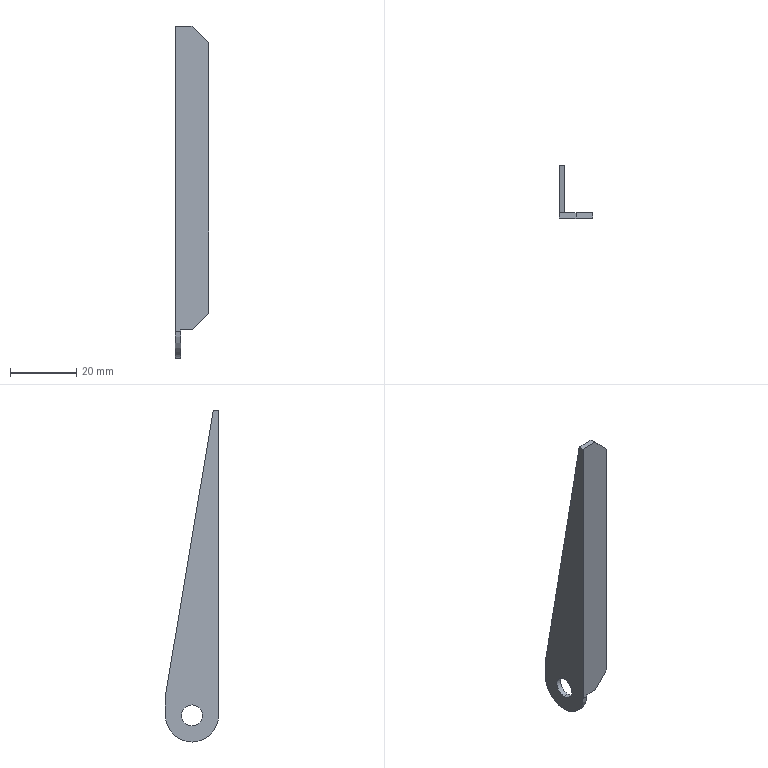Part | SolidWorks | features BaseBody 1 | 1 solid | 15 faces | box 10 x 16 x 100 mm | volume 2664 mm3 | plane 11 | cylinder 4 | commonest cylinder face diameters 6.35 x2 16 x2
STEP:
#1=CARTESIAN_POINT('',(0.,8.,4.825));
#2=VERTEX_POINT('',#1);
#3=CARTESIAN_POINT('',(0.,8.,11.175));
#4=VERTEX_POINT('',#3);
#5=CARTESIAN_POINT('',(0.,8.,8.));
#6=DIRECTION('',(-1.,0.,0.));
#7=DIRECTION('',(0.,0.,-1.));
#8=AXIS2_PLACEMENT_3D('',#5,#6,#7);
#9=CIRCLE('',#8,3.175);
#10=EDGE_CURVE('',#2,#4,#9,.T.);
#11=ORIENTED_EDGE('',*,*,#10,.T.);
#12=CARTESIAN_POINT('',(1.6,8.,11.175));
#13=VERTEX_POINT('',#12);
#14=CARTESIAN_POINT('',(0.,8.,11.175));
#15=DIRECTION('',(1.,0.,0.));
#16=VECTOR('',#15,1000.);
#17=LINE('',#14,#16);
#18=EDGE_CURVE('',#4,#13,#17,.T.);
#19=ORIENTED_EDGE('',*,*,#18,.T.);
#20=CARTESIAN_POINT('',(1.6,8.,4.825));
#21=VERTEX_POINT('',#20);
#22=CARTESIAN_POINT('',(1.6,8.,8.));
#23=DIRECTION('',(1.,0.,0.));
#24=DIRECTION('',(0.,0.,-1.));
#25=AXIS2_PLACEMENT_3D('',#22,#23,#24);
#26=CIRCLE('',#25,3.175);
#27=EDGE_CURVE('',#13,#21,#26,.T.);
#28=ORIENTED_EDGE('',*,*,#27,.T.);
#29=CARTESIAN_POINT('',(0.,8.,4.825));
#30=DIRECTION('',(1.,0.,0.));
#31=VECTOR('',#30,1000.);
#32=LINE('',#29,#31);
#33=EDGE_CURVE('',#2,#21,#32,.T.);
#34=ORIENTED_EDGE('',*,*,#33,.F.);
#35=EDGE_LOOP('',(#11,#19,#28,#34));
#36=FACE_OUTER_BOUND('',#35,.T.);
#37=CARTESIAN_POINT('',(0.,8.,8.));
#38=DIRECTION('',(1.,0.,0.));
#39=DIRECTION('',(0.,0.,-1.));
#40=AXIS2_PLACEMENT_3D('',#37,#38,#39);
#41=CYLINDRICAL_SURFACE('',#40,3.175);
#42=ADVANCED_FACE('',(#36),#41,.F.);
#43=CARTESIAN_POINT('',(0.,0.,8.));
#44=VERTEX_POINT('',#43);
#45=CARTESIAN_POINT('',(0.,8.,0.));
#46=VERTEX_POINT('',#45);
#47=CARTESIAN_POINT('',(0.,8.,8.));
#48=DIRECTION('',(1.,0.,0.));
#49=DIRECTION('',(0.,0.,-1.));
#50=AXIS2_PLACEMENT_3D('',#47,#48,#49);
#51=CIRCLE('',#50,8.);
#52=EDGE_CURVE('',#44,#46,#51,.T.);
#53=ORIENTED_EDGE('',*,*,#52,.T.);
#54=CARTESIAN_POINT('',(1.6,8.,0.));
#55=VERTEX_POINT('',#54);
#56=CARTESIAN_POINT('',(0.,8.,0.));
#57=DIRECTION('',(1.,0.,0.));
#58=VECTOR('',#57,1000.);
#59=LINE('',#56,#58);
#60=EDGE_CURVE('',#46,#55,#59,.T.);
#61=ORIENTED_EDGE('',*,*,#60,.T.);
#62=CARTESIAN_POINT('',(1.6,0.,8.));
#63=VERTEX_POINT('',#62);
#64=CARTESIAN_POINT('',(1.6,8.,8.));
#65=DIRECTION('',(-1.,0.,0.));
#66=DIRECTION('',(0.,0.,-1.));
#67=AXIS2_PLACEMENT_3D('',#64,#65,#66);
#68=CIRCLE('',#67,8.);
#69=EDGE_CURVE('',#55,#63,#68,.T.);
#70=ORIENTED_EDGE('',*,*,#69,.T.);
#71=CARTESIAN_POINT('',(0.8,0.,8.));
#72=DIRECTION('',(1.,0.,0.));
#73=VECTOR('',#72,1000.);
#74=LINE('',#71,#73);
#75=EDGE_CURVE('',#44,#63,#74,.T.);
#76=ORIENTED_EDGE('',*,*,#75,.F.);
#77=EDGE_LOOP('',(#53,#61,#70,#76));
#78=FACE_OUTER_BOUND('',#77,.T.);
#79=CARTESIAN_POINT('',(0.,8.,8.));
#80=DIRECTION('',(1.,0.,0.));
#81=DIRECTION('',(0.,0.,-1.));
#82=AXIS2_PLACEMENT_3D('',#79,#80,#81);
#83=CYLINDRICAL_SURFACE('',#82,8.);
#84=ADVANCED_FACE('',(#78),#83,.T.);
#85=ORIENTED_EDGE('',*,*,#18,.F.);
#86=CARTESIAN_POINT('',(0.,8.,8.));
#87=DIRECTION('',(-1.,0.,0.));
#88=DIRECTION('',(0.,0.,-1.));
#89=AXIS2_PLACEMENT_3D('',#86,#87,#88);
#90=CIRCLE('',#89,3.175);
#91=EDGE_CURVE('',#4,#2,#90,.T.);
#92=ORIENTED_EDGE('',*,*,#91,.T.);
#93=ORIENTED_EDGE('',*,*,#33,.T.);
#94=CARTESIAN_POINT('',(1.6,8.,8.));
#95=DIRECTION('',(1.,0.,0.));
#96=DIRECTION('',(0.,0.,-1.));
#97=AXIS2_PLACEMENT_3D('',#94,#95,#96);
#98=CIRCLE('',#97,3.175);
#99=EDGE_CURVE('',#21,#13,#98,.T.);
#100=ORIENTED_EDGE('',*,*,#99,.T.);
#101=EDGE_LOOP('',(#85,#92,#93,#100));
#102=FACE_OUTER_BOUND('',#101,.T.);
#103=CARTESIAN_POINT('',(0.,8.,8.));
#104=DIRECTION('',(1.,0.,0.));
#105=DIRECTION('',(0.,0.,-1.));
#106=AXIS2_PLACEMENT_3D('',#103,#104,#105);
#107=CYLINDRICAL_SURFACE('',#106,3.175);
#108=ADVANCED_FACE('',(#102),#107,.F.);
#109=ORIENTED_EDGE('',*,*,#99,.F.);
#110=ORIENTED_EDGE('',*,*,#27,.F.);
#111=EDGE_LOOP('',(#109,#110));
#112=FACE_BOUND('',#111,.T.);
#113=CARTESIAN_POINT('',(1.6,1.6,8.502));
#114=VERTEX_POINT('',#113);
#115=CARTESIAN_POINT('',(1.6,0.,8.502));
#116=VERTEX_POINT('',#115);
#117=CARTESIAN_POINT('',(1.6,0.8,8.502));
#118=DIRECTION('',(0.,-1.,0.));
#119=VECTOR('',#118,1000.);
#120=LINE('',#117,#119);
#121=EDGE_CURVE('',#114,#116,#120,.T.);
#122=ORIENTED_EDGE('',*,*,#121,.T.);
#123=CARTESIAN_POINT('',(1.6,0.,54.));
#124=DIRECTION('',(0.,0.,-1.));
#125=VECTOR('',#124,1000.);
#126=LINE('',#123,#125);
#127=EDGE_CURVE('',#116,#63,#126,.T.);
#128=ORIENTED_EDGE('',*,*,#127,.T.);
#129=ORIENTED_EDGE('',*,*,#69,.F.);
#130=CARTESIAN_POINT('',(1.6,16.,8.));
#131=VERTEX_POINT('',#130);
#132=CARTESIAN_POINT('',(1.6,8.,8.));
#133=DIRECTION('',(-1.,0.,0.));
#134=DIRECTION('',(0.,0.,-1.));
#135=AXIS2_PLACEMENT_3D('',#132,#133,#134);
#136=CIRCLE('',#135,8.);
#137=EDGE_CURVE('',#131,#55,#136,.T.);
#138=ORIENTED_EDGE('',*,*,#137,.F.);
#139=CARTESIAN_POINT('',(1.6,16.,14.));
#140=VERTEX_POINT('',#139);
#141=CARTESIAN_POINT('',(1.6,16.,50.));
#142=DIRECTION('',(0.,0.,-1.));
#143=VECTOR('',#142,1000.);
#144=LINE('',#141,#143);
#145=EDGE_CURVE('',#140,#131,#144,.T.);
#146=ORIENTED_EDGE('',*,*,#145,.F.);
#147=CARTESIAN_POINT('',(1.6,1.6,100.));
#148=VERTEX_POINT('',#147);
#149=CARTESIAN_POINT('',(1.6,1.6,100.));
#150=DIRECTION('',(0.,0.1651,-0.9863));
#151=VECTOR('',#150,1000.);
#152=LINE('',#149,#151);
#153=EDGE_CURVE('',#148,#140,#152,.T.);
#154=ORIENTED_EDGE('',*,*,#153,.F.);
#155=CARTESIAN_POINT('',(1.6,1.6,50.));
#156=DIRECTION('',(0.,0.,1.));
#157=VECTOR('',#156,1000.);
#158=LINE('',#155,#157);
#159=EDGE_CURVE('',#114,#148,#158,.T.);
#160=ORIENTED_EDGE('',*,*,#159,.F.);
#161=EDGE_LOOP('',(#122,#128,#129,#138,#146,#154,#160));
#162=FACE_OUTER_BOUND('',#161,.T.);
#163=CARTESIAN_POINT('',(1.6,0.,-0.6));
#164=DIRECTION('',(-1.,0.,0.));
#165=DIRECTION('',(0.,0.,1.));
#166=AXIS2_PLACEMENT_3D('',#163,#164,#165);
#167=PLANE('',#166);
#168=ADVANCED_FACE('',(#112,#162),#167,.F.);
#169=ORIENTED_EDGE('',*,*,#10,.F.);
#170=ORIENTED_EDGE('',*,*,#91,.F.);
#171=EDGE_LOOP('',(#169,#170));
#172=FACE_BOUND('',#171,.T.);
#173=ORIENTED_EDGE('',*,*,#52,.F.);
#174=CARTESIAN_POINT('',(0.,0.,100.));
#175=VERTEX_POINT('',#174);
#176=CARTESIAN_POINT('',(0.,0.,49.7));
#177=DIRECTION('',(0.,0.,-1.));
#178=VECTOR('',#177,1000.);
#179=LINE('',#176,#178);
#180=EDGE_CURVE('',#175,#44,#179,.T.);
#181=ORIENTED_EDGE('',*,*,#180,.F.);
#182=CARTESIAN_POINT('',(0.,1.6,100.));
#183=VERTEX_POINT('',#182);
#184=CARTESIAN_POINT('',(0.,0.8,100.));
#185=DIRECTION('',(0.,1.,0.));
#186=VECTOR('',#185,1000.);
#187=LINE('',#184,#186);
#188=EDGE_CURVE('',#175,#183,#187,.T.);
#189=ORIENTED_EDGE('',*,*,#188,.T.);
#190=CARTESIAN_POINT('',(0.,16.,14.));
#191=VERTEX_POINT('',#190);
#192=CARTESIAN_POINT('',(0.,1.6,100.));
#193=DIRECTION('',(0.,-0.1651,0.9863));
#194=VECTOR('',#193,1000.);
#195=LINE('',#192,#194);
#196=EDGE_CURVE('',#191,#183,#195,.T.);
#197=ORIENTED_EDGE('',*,*,#196,.F.);
#198=CARTESIAN_POINT('',(0.,16.,8.));
#199=VERTEX_POINT('',#198);
#200=CARTESIAN_POINT('',(0.,16.,49.7));
#201=DIRECTION('',(0.,0.,1.));
#202=VECTOR('',#201,1000.);
#203=LINE('',#200,#202);
#204=EDGE_CURVE('',#199,#191,#203,.T.);
#205=ORIENTED_EDGE('',*,*,#204,.F.);
#206=CARTESIAN_POINT('',(0.,8.,8.));
#207=DIRECTION('',(1.,0.,0.));
#208=DIRECTION('',(0.,0.,-1.));
#209=AXIS2_PLACEMENT_3D('',#206,#207,#208);
#210=CIRCLE('',#209,8.);
#211=EDGE_CURVE('',#46,#199,#210,.T.);
#212=ORIENTED_EDGE('',*,*,#211,.F.);
#213=EDGE_LOOP('',(#173,#181,#189,#197,#205,#212));
#214=FACE_OUTER_BOUND('',#213,.T.);
#215=CARTESIAN_POINT('',(0.,0.,-0.6));
#216=DIRECTION('',(1.,0.,0.));
#217=DIRECTION('',(0.,1.,0.));
#218=AXIS2_PLACEMENT_3D('',#215,#216,#217);
#219=PLANE('',#218);
#220=ADVANCED_FACE('',(#172,#214),#219,.F.);
#221=CARTESIAN_POINT('',(5.,1.6,8.502));
#222=VERTEX_POINT('',#221);
#223=CARTESIAN_POINT('',(10.,1.6,13.502));
#224=VERTEX_POINT('',#223);
#225=CARTESIAN_POINT('',(5.,1.6,8.502));
#226=DIRECTION('',(0.7071,0.,0.7071));
#227=VECTOR('',#226,1000.);
#228=LINE('',#225,#227);
#229=EDGE_CURVE('',#222,#224,#228,.T.);
#230=ORIENTED_EDGE('',*,*,#229,.F.);
#231=CARTESIAN_POINT('',(5.8,1.6,8.502));
#232=DIRECTION('',(1.,0.,0.));
#233=VECTOR('',#232,1000.);
#234=LINE('',#231,#233);
#235=EDGE_CURVE('',#114,#222,#234,.T.);
#236=ORIENTED_EDGE('',*,*,#235,.F.);
#237=ORIENTED_EDGE('',*,*,#159,.T.);
#238=CARTESIAN_POINT('',(5.,1.6,100.));
#239=VERTEX_POINT('',#238);
#240=CARTESIAN_POINT('',(5.8,1.6,100.));
#241=DIRECTION('',(-1.,0.,0.));
#242=VECTOR('',#241,1000.);
#243=LINE('',#240,#242);
#244=EDGE_CURVE('',#239,#148,#243,.T.);
#245=ORIENTED_EDGE('',*,*,#244,.F.);
#246=CARTESIAN_POINT('',(10.,1.6,95.));
#247=VERTEX_POINT('',#246);
#248=CARTESIAN_POINT('',(10.,1.6,95.));
#249=DIRECTION('',(-0.7071,0.,0.7071));
#250=VECTOR('',#249,1000.);
#251=LINE('',#248,#250);
#252=EDGE_CURVE('',#247,#239,#251,.T.);
#253=ORIENTED_EDGE('',*,*,#252,.F.);
#254=CARTESIAN_POINT('',(10.,1.6,54.251));
#255=DIRECTION('',(0.,0.,1.));
#256=VECTOR('',#255,1000.);
#257=LINE('',#254,#256);
#258=EDGE_CURVE('',#224,#247,#257,.T.);
#259=ORIENTED_EDGE('',*,*,#258,.F.);
#260=EDGE_LOOP('',(#230,#236,#237,#245,#253,#259));
#261=FACE_OUTER_BOUND('',#260,.T.);
#262=CARTESIAN_POINT('',(1.6,1.6,100.));
#263=DIRECTION('',(0.,-1.,0.));
#264=DIRECTION('',(0.,0.,-1.));
#265=AXIS2_PLACEMENT_3D('',#262,#263,#264);
#266=PLANE('',#265);
#267=ADVANCED_FACE('',(#261),#266,.F.);
#268=ORIENTED_EDGE('',*,*,#60,.F.);
#269=ORIENTED_EDGE('',*,*,#211,.T.);
#270=CARTESIAN_POINT('',(0.8,16.,8.));
#271=DIRECTION('',(-1.,0.,0.));
#272=VECTOR('',#271,1000.);
#273=LINE('',#270,#272);
#274=EDGE_CURVE('',#131,#199,#273,.T.);
#275=ORIENTED_EDGE('',*,*,#274,.F.);
#276=ORIENTED_EDGE('',*,*,#137,.T.);
#277=EDGE_LOOP('',(#268,#269,#275,#276));
#278=FACE_OUTER_BOUND('',#277,.T.);
#279=CARTESIAN_POINT('',(0.,8.,8.));
#280=DIRECTION('',(1.,0.,0.));
#281=DIRECTION('',(0.,0.,-1.));
#282=AXIS2_PLACEMENT_3D('',#279,#280,#281);
#283=CYLINDRICAL_SURFACE('',#282,8.);
#284=ADVANCED_FACE('',(#278),#283,.T.);
#285=ORIENTED_EDGE('',*,*,#274,.T.);
#286=ORIENTED_EDGE('',*,*,#204,.T.);
#287=CARTESIAN_POINT('',(0.8,16.,14.));
#288=DIRECTION('',(-1.,0.,0.));
#289=VECTOR('',#288,1000.);
#290=LINE('',#287,#289);
#291=EDGE_CURVE('',#140,#191,#290,.T.);
#292=ORIENTED_EDGE('',*,*,#291,.F.);
#293=ORIENTED_EDGE('',*,*,#145,.T.);
#294=EDGE_LOOP('',(#285,#286,#292,#293));
#295=FACE_OUTER_BOUND('',#294,.T.);
#296=CARTESIAN_POINT('',(0.,16.,14.));
#297=DIRECTION('',(0.,-1.,0.));
#298=DIRECTION('',(0.,0.,-1.));
#299=AXIS2_PLACEMENT_3D('',#296,#297,#298);
#300=PLANE('',#299);
#301=ADVANCED_FACE('',(#295),#300,.F.);
#302=ORIENTED_EDGE('',*,*,#153,.T.);
#303=ORIENTED_EDGE('',*,*,#291,.T.);
#304=ORIENTED_EDGE('',*,*,#196,.T.);
#305=CARTESIAN_POINT('',(0.8,1.6,100.));
#306=DIRECTION('',(-1.,0.,0.));
#307=VECTOR('',#306,1000.);
#308=LINE('',#305,#307);
#309=EDGE_CURVE('',#148,#183,#308,.T.);
#310=ORIENTED_EDGE('',*,*,#309,.F.);
#311=EDGE_LOOP('',(#302,#303,#304,#310));
#312=FACE_OUTER_BOUND('',#311,.T.);
#313=CARTESIAN_POINT('',(0.,1.6,100.));
#314=DIRECTION('',(0.,-0.9863,-0.1651));
#315=DIRECTION('',(0.,0.1651,-0.9863));
#316=AXIS2_PLACEMENT_3D('',#313,#314,#315);
#317=PLANE('',#316);
#318=ADVANCED_FACE('',(#312),#317,.F.);
#319=CARTESIAN_POINT('',(10.,0.,13.502));
#320=VERTEX_POINT('',#319);
#321=CARTESIAN_POINT('',(5.,0.,8.502));
#322=VERTEX_POINT('',#321);
#323=CARTESIAN_POINT('',(5.,0.,8.502));
#324=DIRECTION('',(-0.7071,0.,-0.7071));
#325=VECTOR('',#324,1000.);
#326=LINE('',#323,#325);
#327=EDGE_CURVE('',#320,#322,#326,.T.);
#328=ORIENTED_EDGE('',*,*,#327,.F.);
#329=CARTESIAN_POINT('',(10.,0.,95.));
#330=VERTEX_POINT('',#329);
#331=CARTESIAN_POINT('',(10.,0.,54.));
#332=DIRECTION('',(0.,0.,-1.));
#333=VECTOR('',#332,1000.);
#334=LINE('',#331,#333);
#335=EDGE_CURVE('',#330,#320,#334,.T.);
#336=ORIENTED_EDGE('',*,*,#335,.F.);
#337=CARTESIAN_POINT('',(5.,0.,100.));
#338=VERTEX_POINT('',#337);
#339=CARTESIAN_POINT('',(10.,0.,95.));
#340=DIRECTION('',(0.7071,0.,-0.7071));
#341=VECTOR('',#340,1000.);
#342=LINE('',#339,#341);
#343=EDGE_CURVE('',#338,#330,#342,.T.);
#344=ORIENTED_EDGE('',*,*,#343,.F.);
#345=CARTESIAN_POINT('',(5.,0.,100.));
#346=DIRECTION('',(1.,0.,0.));
#347=VECTOR('',#346,1000.);
#348=LINE('',#345,#347);
#349=EDGE_CURVE('',#175,#338,#348,.T.);
#350=ORIENTED_EDGE('',*,*,#349,.F.);
#351=ORIENTED_EDGE('',*,*,#180,.T.);
#352=ORIENTED_EDGE('',*,*,#75,.T.);
#353=ORIENTED_EDGE('',*,*,#127,.F.);
#354=CARTESIAN_POINT('',(5.,0.,8.502));
#355=DIRECTION('',(-1.,0.,0.));
#356=VECTOR('',#355,1000.);
#357=LINE('',#354,#356);
#358=EDGE_CURVE('',#322,#116,#357,.T.);
#359=ORIENTED_EDGE('',*,*,#358,.F.);
#360=EDGE_LOOP('',(#328,#336,#344,#350,#351,#352,#353,#359));
#361=FACE_OUTER_BOUND('',#360,.T.);
#362=CARTESIAN_POINT('',(0.,0.,8.));
#363=DIRECTION('',(0.,1.,0.));
#364=DIRECTION('',(0.,0.,1.));
#365=AXIS2_PLACEMENT_3D('',#362,#363,#364);
#366=PLANE('',#365);
#367=ADVANCED_FACE('',(#361),#366,.F.);
#368=CARTESIAN_POINT('',(10.,0.8,13.502));
#369=DIRECTION('',(0.,-1.,0.));
#370=VECTOR('',#369,1000.);
#371=LINE('',#368,#370);
#372=EDGE_CURVE('',#224,#320,#371,.T.);
#373=ORIENTED_EDGE('',*,*,#372,.F.);
#374=ORIENTED_EDGE('',*,*,#258,.T.);
#375=CARTESIAN_POINT('',(10.,0.8,95.));
#376=DIRECTION('',(0.,1.,0.));
#377=VECTOR('',#376,1000.);
#378=LINE('',#375,#377);
#379=EDGE_CURVE('',#330,#247,#378,.T.);
#380=ORIENTED_EDGE('',*,*,#379,.F.);
#381=ORIENTED_EDGE('',*,*,#335,.T.);
#382=EDGE_LOOP('',(#373,#374,#380,#381));
#383=FACE_OUTER_BOUND('',#382,.T.);
#384=CARTESIAN_POINT('',(10.,0.,13.502));
#385=DIRECTION('',(-1.,0.,0.));
#386=DIRECTION('',(0.,0.,1.));
#387=AXIS2_PLACEMENT_3D('',#384,#385,#386);
#388=PLANE('',#387);
#389=ADVANCED_FACE('',(#383),#388,.F.);
#390=CARTESIAN_POINT('',(5.,0.8,8.502));
#391=DIRECTION('',(0.,-1.,0.));
#392=VECTOR('',#391,1000.);
#393=LINE('',#390,#392);
#394=EDGE_CURVE('',#222,#322,#393,.T.);
#395=ORIENTED_EDGE('',*,*,#394,.F.);
#396=ORIENTED_EDGE('',*,*,#229,.T.);
#397=ORIENTED_EDGE('',*,*,#372,.T.);
#398=ORIENTED_EDGE('',*,*,#327,.T.);
#399=EDGE_LOOP('',(#395,#396,#397,#398));
#400=FACE_OUTER_BOUND('',#399,.T.);
#401=CARTESIAN_POINT('',(5.,0.,8.502));
#402=DIRECTION('',(-0.7071,0.,0.7071));
#403=DIRECTION('',(0.7071,0.,0.7071));
#404=AXIS2_PLACEMENT_3D('',#401,#402,#403);
#405=PLANE('',#404);
#406=ADVANCED_FACE('',(#400),#405,.F.);
#407=ORIENTED_EDGE('',*,*,#394,.T.);
#408=ORIENTED_EDGE('',*,*,#358,.T.);
#409=ORIENTED_EDGE('',*,*,#121,.F.);
#410=ORIENTED_EDGE('',*,*,#235,.T.);
#411=EDGE_LOOP('',(#407,#408,#409,#410));
#412=FACE_OUTER_BOUND('',#411,.T.);
#413=CARTESIAN_POINT('',(1.6,0.,8.502));
#414=DIRECTION('',(0.,0.,1.));
#415=DIRECTION('',(1.,0.,0.));
#416=AXIS2_PLACEMENT_3D('',#413,#414,#415);
#417=PLANE('',#416);
#418=ADVANCED_FACE('',(#412),#417,.F.);
#419=ORIENTED_EDGE('',*,*,#309,.T.);
#420=ORIENTED_EDGE('',*,*,#188,.F.);
#421=ORIENTED_EDGE('',*,*,#349,.T.);
#422=CARTESIAN_POINT('',(5.,0.8,100.));
#423=DIRECTION('',(0.,-1.,0.));
#424=VECTOR('',#423,1000.);
#425=LINE('',#422,#424);
#426=EDGE_CURVE('',#239,#338,#425,.T.);
#427=ORIENTED_EDGE('',*,*,#426,.F.);
#428=ORIENTED_EDGE('',*,*,#244,.T.);
#429=EDGE_LOOP('',(#419,#420,#421,#427,#428));
#430=FACE_OUTER_BOUND('',#429,.T.);
#431=CARTESIAN_POINT('',(5.,0.,100.));
#432=DIRECTION('',(0.,0.,-1.));
#433=DIRECTION('',(-1.,0.,0.));
#434=AXIS2_PLACEMENT_3D('',#431,#432,#433);
#435=PLANE('',#434);
#436=ADVANCED_FACE('',(#430),#435,.F.);
#437=ORIENTED_EDGE('',*,*,#379,.T.);
#438=ORIENTED_EDGE('',*,*,#252,.T.);
#439=ORIENTED_EDGE('',*,*,#426,.T.);
#440=ORIENTED_EDGE('',*,*,#343,.T.);
#441=EDGE_LOOP('',(#437,#438,#439,#440));
#442=FACE_OUTER_BOUND('',#441,.T.);
#443=CARTESIAN_POINT('',(10.,0.,95.));
#444=DIRECTION('',(-0.7071,0.,-0.7071));
#445=DIRECTION('',(-0.7071,0.,0.7071));
#446=AXIS2_PLACEMENT_3D('',#443,#444,#445);
#447=PLANE('',#446);
#448=ADVANCED_FACE('',(#442),#447,.F.);
#449=CLOSED_SHELL('',(#42,#84,#108,#168,#220,#267,#284,#301,#318,#367,#389,#406,#418,#436,#448));
#450=MANIFOLD_SOLID_BREP('',#449);
#451=CARTESIAN_POINT('',(0.,0.,0.));
#452=DIRECTION('',(0.,0.,1.));
#453=DIRECTION('',(1.,0.,0.));
#454=AXIS2_PLACEMENT_3D('',#451,#452,#453);
#455=(LENGTH_UNIT()NAMED_UNIT(*)SI_UNIT(.MILLI.,.METRE.));
#456=UNCERTAINTY_MEASURE_WITH_UNIT(LENGTH_MEASURE(0.00001),#455,'','');
#457=(NAMED_UNIT(*)PLANE_ANGLE_UNIT()SI_UNIT($,.RADIAN.));
#458=(NAMED_UNIT(*)SI_UNIT($,.STERADIAN.)SOLID_ANGLE_UNIT());
#459=(GEOMETRIC_REPRESENTATION_CONTEXT(3)GLOBAL_UNCERTAINTY_ASSIGNED_CONTEXT((#456))GLOBAL_UNIT_ASSIGNED_CONTEXT((#455,#457,#458))REPRESENTATION_CONTEXT('',''));
#460=ADVANCED_BREP_SHAPE_REPRESENTATION('',(#450,#454),#459);